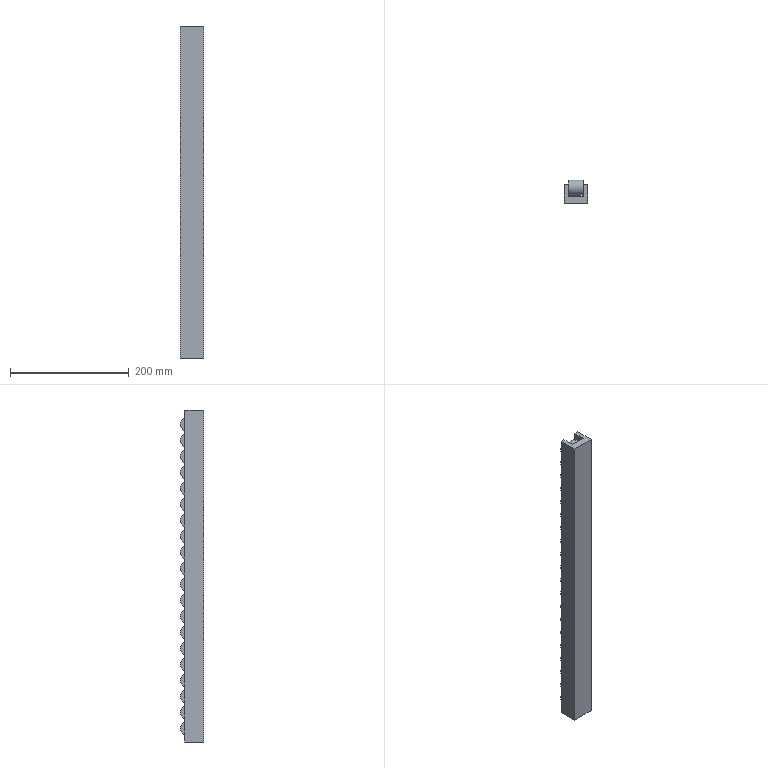Part | STEP file | PN_0069 wheel-type conveyor belt | 1 solid | 90 faces | box 40 x 39.5 x 560 mm | volume 671037 mm3 | plane 50 | cylinder 40 | commonest cylinder face diameters 25 x40